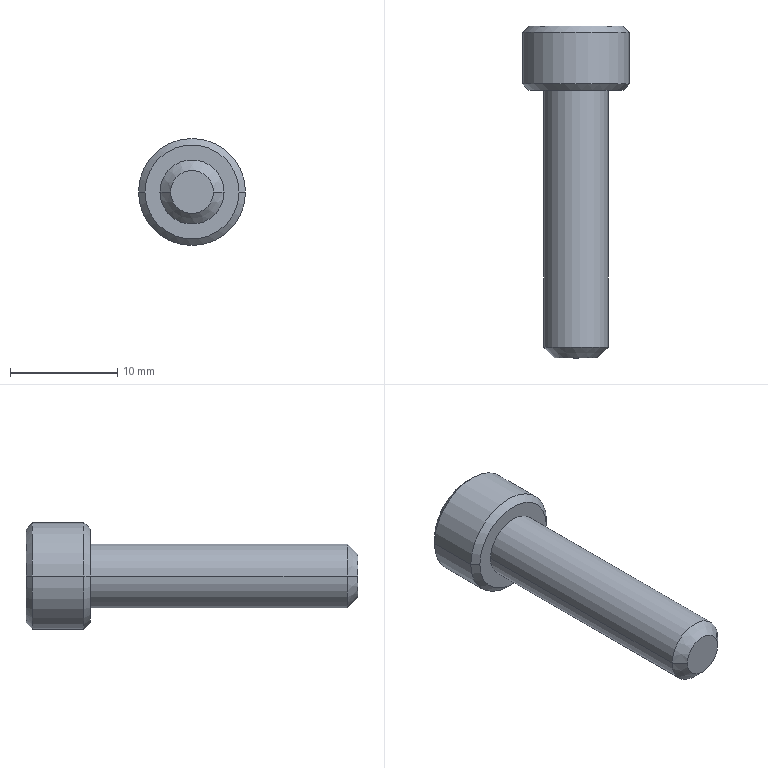Part | STEP file | BB62-M6-25L-1 | 1 solid | 27 faces | box 10 x 31 x 10 mm | volume 1081 mm3 | plane 15 | cone 8 | cylinder 4 | commonest cylinder face diameters 6 x2 10 x2
STEP:
#1=CARTESIAN_POINT('',(0.,1.349,0.));
#2=VERTEX_POINT('',#1);
#3=CARTESIAN_POINT('',(2.86,3.,0.));
#4=VERTEX_POINT('',#3);
#5=CARTESIAN_POINT('',(0.,1.349,0.));
#6=DIRECTION('',(0.866,0.5,0.));
#7=VECTOR('',#6,1000.);
#8=LINE('',#5,#7);
#9=EDGE_CURVE('',#2,#4,#8,.T.);
#10=ORIENTED_EDGE('',*,*,#9,.F.);
#11=CARTESIAN_POINT('',(-2.86,3.,0.));
#12=VERTEX_POINT('',#11);
#13=CARTESIAN_POINT('',(0.,1.349,0.));
#14=DIRECTION('',(-0.866,0.5,0.));
#15=VECTOR('',#14,1000.);
#16=LINE('',#13,#15);
#17=EDGE_CURVE('',#2,#12,#16,.T.);
#18=ORIENTED_EDGE('',*,*,#17,.T.);
#19=CARTESIAN_POINT('',(-2.477,3.,1.43));
#20=VERTEX_POINT('',#19);
#21=CARTESIAN_POINT('',(0.,3.,0.));
#22=DIRECTION('',(0.,-1.,0.));
#23=DIRECTION('',(-1.,0.,0.));
#24=AXIS2_PLACEMENT_3D('',#21,#22,#23);
#25=CIRCLE('',#24,2.86);
#26=EDGE_CURVE('',#20,#12,#25,.T.);
#27=ORIENTED_EDGE('',*,*,#26,.F.);
#28=CARTESIAN_POINT('',(0.,3.,2.86));
#29=VERTEX_POINT('',#28);
#30=CARTESIAN_POINT('',(0.,3.,0.));
#31=DIRECTION('',(0.,-1.,0.));
#32=DIRECTION('',(-1.,0.,0.));
#33=AXIS2_PLACEMENT_3D('',#30,#31,#32);
#34=CIRCLE('',#33,2.86);
#35=EDGE_CURVE('',#29,#20,#34,.T.);
#36=ORIENTED_EDGE('',*,*,#35,.F.);
#37=CARTESIAN_POINT('',(2.477,3.,1.43));
#38=VERTEX_POINT('',#37);
#39=CARTESIAN_POINT('',(0.,3.,0.));
#40=DIRECTION('',(0.,-1.,0.));
#41=DIRECTION('',(-1.,0.,0.));
#42=AXIS2_PLACEMENT_3D('',#39,#40,#41);
#43=CIRCLE('',#42,2.86);
#44=EDGE_CURVE('',#38,#29,#43,.T.);
#45=ORIENTED_EDGE('',*,*,#44,.F.);
#46=CARTESIAN_POINT('',(0.,3.,0.));
#47=DIRECTION('',(0.,-1.,0.));
#48=DIRECTION('',(-1.,0.,0.));
#49=AXIS2_PLACEMENT_3D('',#46,#47,#48);
#50=CIRCLE('',#49,2.86);
#51=EDGE_CURVE('',#4,#38,#50,.T.);
#52=ORIENTED_EDGE('',*,*,#51,.F.);
#53=EDGE_LOOP('',(#10,#18,#27,#36,#45,#52));
#54=FACE_OUTER_BOUND('',#53,.T.);
#55=CARTESIAN_POINT('',(0.,1001.349,0.));
#56=DIRECTION('',(0.,1.,0.));
#57=DIRECTION('',(1.,0.,0.));
#58=AXIS2_PLACEMENT_3D('',#55,#56,#57);
#59=CONICAL_SURFACE('',#58,1732.051,1.047);
#60=ADVANCED_FACE('',(#54),#59,.F.);
#61=CARTESIAN_POINT('',(2.,-25.,0.));
#62=VERTEX_POINT('',#61);
#63=CARTESIAN_POINT('',(-2.,-25.,0.));
#64=VERTEX_POINT('',#63);
#65=CARTESIAN_POINT('',(0.,-25.,0.));
#66=DIRECTION('',(0.,1.,0.));
#67=DIRECTION('',(1.,0.,0.));
#68=AXIS2_PLACEMENT_3D('',#65,#66,#67);
#69=CIRCLE('',#68,2.);
#70=EDGE_CURVE('',#62,#64,#69,.T.);
#71=ORIENTED_EDGE('',*,*,#70,.T.);
#72=CARTESIAN_POINT('',(-3.,-24.,0.));
#73=VERTEX_POINT('',#72);
#74=CARTESIAN_POINT('',(-2.,-25.,0.));
#75=DIRECTION('',(-0.7071,0.7071,0.));
#76=VECTOR('',#75,1000.);
#77=LINE('',#74,#76);
#78=EDGE_CURVE('',#64,#73,#77,.T.);
#79=ORIENTED_EDGE('',*,*,#78,.T.);
#80=CARTESIAN_POINT('',(3.,-24.,0.));
#81=VERTEX_POINT('',#80);
#82=CARTESIAN_POINT('',(0.,-24.,0.));
#83=DIRECTION('',(0.,-1.,0.));
#84=DIRECTION('',(-1.,0.,0.));
#85=AXIS2_PLACEMENT_3D('',#82,#83,#84);
#86=CIRCLE('',#85,3.);
#87=EDGE_CURVE('',#73,#81,#86,.T.);
#88=ORIENTED_EDGE('',*,*,#87,.T.);
#89=CARTESIAN_POINT('',(2.,-25.,0.));
#90=DIRECTION('',(0.7071,0.7071,0.));
#91=VECTOR('',#90,1000.);
#92=LINE('',#89,#91);
#93=EDGE_CURVE('',#62,#81,#92,.T.);
#94=ORIENTED_EDGE('',*,*,#93,.F.);
#95=EDGE_LOOP('',(#71,#79,#88,#94));
#96=FACE_OUTER_BOUND('',#95,.T.);
#97=CARTESIAN_POINT('',(0.,-25.,0.));
#98=DIRECTION('',(0.,1.,0.));
#99=DIRECTION('',(1.,0.,0.));
#100=AXIS2_PLACEMENT_3D('',#97,#98,#99);
#101=CONICAL_SURFACE('',#100,2.,0.7854);
#102=ADVANCED_FACE('',(#96),#101,.T.);
#103=ORIENTED_EDGE('',*,*,#87,.F.);
#104=CARTESIAN_POINT('',(-3.,0.,0.));
#105=VERTEX_POINT('',#104);
#106=CARTESIAN_POINT('',(-3.,-24.,0.));
#107=DIRECTION('',(0.,1.,0.));
#108=VECTOR('',#107,1000.);
#109=LINE('',#106,#108);
#110=EDGE_CURVE('',#73,#105,#109,.T.);
#111=ORIENTED_EDGE('',*,*,#110,.T.);
#112=CARTESIAN_POINT('',(3.,0.,0.));
#113=VERTEX_POINT('',#112);
#114=CARTESIAN_POINT('',(0.,0.,0.));
#115=DIRECTION('',(0.,-1.,0.));
#116=DIRECTION('',(-1.,0.,0.));
#117=AXIS2_PLACEMENT_3D('',#114,#115,#116);
#118=CIRCLE('',#117,3.);
#119=EDGE_CURVE('',#105,#113,#118,.T.);
#120=ORIENTED_EDGE('',*,*,#119,.T.);
#121=CARTESIAN_POINT('',(3.,-24.,0.));
#122=DIRECTION('',(0.,1.,0.));
#123=VECTOR('',#122,1000.);
#124=LINE('',#121,#123);
#125=EDGE_CURVE('',#81,#113,#124,.T.);
#126=ORIENTED_EDGE('',*,*,#125,.F.);
#127=EDGE_LOOP('',(#103,#111,#120,#126));
#128=FACE_OUTER_BOUND('',#127,.T.);
#129=CARTESIAN_POINT('',(0.,-24.,0.));
#130=DIRECTION('',(0.,1.,0.));
#131=DIRECTION('',(1.,0.,0.));
#132=AXIS2_PLACEMENT_3D('',#129,#130,#131);
#133=CYLINDRICAL_SURFACE('',#132,3.);
#134=ADVANCED_FACE('',(#128),#133,.T.);
#135=CARTESIAN_POINT('',(-4.4,6.,0.));
#136=VERTEX_POINT('',#135);
#137=CARTESIAN_POINT('',(4.4,6.,0.));
#138=VERTEX_POINT('',#137);
#139=CARTESIAN_POINT('',(0.,6.,0.));
#140=DIRECTION('',(0.,-1.,0.));
#141=DIRECTION('',(-1.,0.,0.));
#142=AXIS2_PLACEMENT_3D('',#139,#140,#141);
#143=CIRCLE('',#142,4.4);
#144=EDGE_CURVE('',#136,#138,#143,.T.);
#145=ORIENTED_EDGE('',*,*,#144,.T.);
#146=CARTESIAN_POINT('',(5.,5.4,0.));
#147=VERTEX_POINT('',#146);
#148=CARTESIAN_POINT('',(5.,5.4,0.));
#149=DIRECTION('',(0.7071,-0.7071,0.));
#150=VECTOR('',#149,1000.);
#151=LINE('',#148,#150);
#152=EDGE_CURVE('',#138,#147,#151,.T.);
#153=ORIENTED_EDGE('',*,*,#152,.T.);
#154=CARTESIAN_POINT('',(-5.,5.4,0.));
#155=VERTEX_POINT('',#154);
#156=CARTESIAN_POINT('',(0.,5.4,0.));
#157=DIRECTION('',(0.,-1.,0.));
#158=DIRECTION('',(-1.,0.,0.));
#159=AXIS2_PLACEMENT_3D('',#156,#157,#158);
#160=CIRCLE('',#159,5.);
#161=EDGE_CURVE('',#155,#147,#160,.T.);
#162=ORIENTED_EDGE('',*,*,#161,.F.);
#163=CARTESIAN_POINT('',(-5.,5.4,0.));
#164=DIRECTION('',(-0.7071,-0.7071,0.));
#165=VECTOR('',#164,1000.);
#166=LINE('',#163,#165);
#167=EDGE_CURVE('',#136,#155,#166,.T.);
#168=ORIENTED_EDGE('',*,*,#167,.F.);
#169=EDGE_LOOP('',(#145,#153,#162,#168));
#170=FACE_OUTER_BOUND('',#169,.T.);
#171=CARTESIAN_POINT('',(0.,5.4,0.));
#172=DIRECTION('',(0.,-1.,0.));
#173=DIRECTION('',(-1.,0.,0.));
#174=AXIS2_PLACEMENT_3D('',#171,#172,#173);
#175=CONICAL_SURFACE('',#174,5.,0.7854);
#176=ADVANCED_FACE('',(#170),#175,.T.);
#177=ORIENTED_EDGE('',*,*,#161,.T.);
#178=CARTESIAN_POINT('',(5.,0.6,0.));
#179=VERTEX_POINT('',#178);
#180=CARTESIAN_POINT('',(5.,1.62,0.));
#181=DIRECTION('',(0.,-1.,0.));
#182=VECTOR('',#181,1000.);
#183=LINE('',#180,#182);
#184=EDGE_CURVE('',#147,#179,#183,.T.);
#185=ORIENTED_EDGE('',*,*,#184,.T.);
#186=CARTESIAN_POINT('',(-5.,0.6,0.));
#187=VERTEX_POINT('',#186);
#188=CARTESIAN_POINT('',(0.,0.6,0.));
#189=DIRECTION('',(0.,-1.,0.));
#190=DIRECTION('',(-1.,0.,0.));
#191=AXIS2_PLACEMENT_3D('',#188,#189,#190);
#192=CIRCLE('',#191,5.);
#193=EDGE_CURVE('',#187,#179,#192,.T.);
#194=ORIENTED_EDGE('',*,*,#193,.F.);
#195=CARTESIAN_POINT('',(-5.,1.62,0.));
#196=DIRECTION('',(0.,-1.,0.));
#197=VECTOR('',#196,1000.);
#198=LINE('',#195,#197);
#199=EDGE_CURVE('',#155,#187,#198,.T.);
#200=ORIENTED_EDGE('',*,*,#199,.F.);
#201=EDGE_LOOP('',(#177,#185,#194,#200));
#202=FACE_OUTER_BOUND('',#201,.T.);
#203=CARTESIAN_POINT('',(0.,1.62,0.));
#204=DIRECTION('',(0.,-1.,0.));
#205=DIRECTION('',(-1.,0.,0.));
#206=AXIS2_PLACEMENT_3D('',#203,#204,#205);
#207=CYLINDRICAL_SURFACE('',#206,5.);
#208=ADVANCED_FACE('',(#202),#207,.T.);
#209=CARTESIAN_POINT('',(-4.4,0.,0.));
#210=VERTEX_POINT('',#209);
#211=CARTESIAN_POINT('',(4.4,0.,0.));
#212=VERTEX_POINT('',#211);
#213=CARTESIAN_POINT('',(0.,0.,0.));
#214=DIRECTION('',(0.,-1.,0.));
#215=DIRECTION('',(-1.,0.,0.));
#216=AXIS2_PLACEMENT_3D('',#213,#214,#215);
#217=CIRCLE('',#216,4.4);
#218=EDGE_CURVE('',#210,#212,#217,.T.);
#219=ORIENTED_EDGE('',*,*,#218,.F.);
#220=CARTESIAN_POINT('',(-4.4,0.,0.));
#221=DIRECTION('',(-0.7071,0.7071,0.));
#222=VECTOR('',#221,1000.);
#223=LINE('',#220,#222);
#224=EDGE_CURVE('',#210,#187,#223,.T.);
#225=ORIENTED_EDGE('',*,*,#224,.T.);
#226=ORIENTED_EDGE('',*,*,#193,.T.);
#227=CARTESIAN_POINT('',(4.4,0.,0.));
#228=DIRECTION('',(0.7071,0.7071,0.));
#229=VECTOR('',#228,1000.);
#230=LINE('',#227,#229);
#231=EDGE_CURVE('',#212,#179,#230,.T.);
#232=ORIENTED_EDGE('',*,*,#231,.F.);
#233=EDGE_LOOP('',(#219,#225,#226,#232));
#234=FACE_OUTER_BOUND('',#233,.T.);
#235=CARTESIAN_POINT('',(0.,0.,0.));
#236=DIRECTION('',(0.,1.,0.));
#237=DIRECTION('',(1.,0.,0.));
#238=AXIS2_PLACEMENT_3D('',#235,#236,#237);
#239=CONICAL_SURFACE('',#238,4.4,0.7854);
#240=ADVANCED_FACE('',(#234),#239,.T.);
#241=ORIENTED_EDGE('',*,*,#144,.F.);
#242=CARTESIAN_POINT('',(0.,6.,0.));
#243=DIRECTION('',(0.,-1.,0.));
#244=DIRECTION('',(-1.,0.,0.));
#245=AXIS2_PLACEMENT_3D('',#242,#243,#244);
#246=CIRCLE('',#245,4.4);
#247=EDGE_CURVE('',#138,#136,#246,.T.);
#248=ORIENTED_EDGE('',*,*,#247,.F.);
#249=EDGE_LOOP('',(#241,#248));
#250=FACE_OUTER_BOUND('',#249,.T.);
#251=CARTESIAN_POINT('',(0.,6.,-2.86));
#252=VERTEX_POINT('',#251);
#253=CARTESIAN_POINT('',(-2.477,6.,-1.43));
#254=VERTEX_POINT('',#253);
#255=CARTESIAN_POINT('',(0.,6.,-2.86));
#256=DIRECTION('',(-0.866,0.,0.5));
#257=VECTOR('',#256,1000.);
#258=LINE('',#255,#257);
#259=EDGE_CURVE('',#252,#254,#258,.T.);
#260=ORIENTED_EDGE('',*,*,#259,.F.);
#261=CARTESIAN_POINT('',(2.477,6.,-1.43));
#262=VERTEX_POINT('',#261);
#263=CARTESIAN_POINT('',(2.477,6.,-1.43));
#264=DIRECTION('',(-0.866,0.,-0.5));
#265=VECTOR('',#264,1000.);
#266=LINE('',#263,#265);
#267=EDGE_CURVE('',#262,#252,#266,.T.);
#268=ORIENTED_EDGE('',*,*,#267,.F.);
#269=CARTESIAN_POINT('',(2.477,6.,1.43));
#270=VERTEX_POINT('',#269);
#271=CARTESIAN_POINT('',(2.477,6.,1.43));
#272=DIRECTION('',(0.,0.,-1.));
#273=VECTOR('',#272,1000.);
#274=LINE('',#271,#273);
#275=EDGE_CURVE('',#270,#262,#274,.T.);
#276=ORIENTED_EDGE('',*,*,#275,.F.);
#277=CARTESIAN_POINT('',(0.,6.,2.86));
#278=VERTEX_POINT('',#277);
#279=CARTESIAN_POINT('',(0.,6.,2.86));
#280=DIRECTION('',(0.866,0.,-0.5));
#281=VECTOR('',#280,1000.);
#282=LINE('',#279,#281);
#283=EDGE_CURVE('',#278,#270,#282,.T.);
#284=ORIENTED_EDGE('',*,*,#283,.F.);
#285=CARTESIAN_POINT('',(-2.477,6.,1.43));
#286=VERTEX_POINT('',#285);
#287=CARTESIAN_POINT('',(-2.477,6.,1.43));
#288=DIRECTION('',(0.866,0.,0.5));
#289=VECTOR('',#288,1000.);
#290=LINE('',#287,#289);
#291=EDGE_CURVE('',#286,#278,#290,.T.);
#292=ORIENTED_EDGE('',*,*,#291,.F.);
#293=CARTESIAN_POINT('',(-2.477,6.,-1.43));
#294=DIRECTION('',(0.,0.,1.));
#295=VECTOR('',#294,1000.);
#296=LINE('',#293,#295);
#297=EDGE_CURVE('',#254,#286,#296,.T.);
#298=ORIENTED_EDGE('',*,*,#297,.F.);
#299=EDGE_LOOP('',(#260,#268,#276,#284,#292,#298));
#300=FACE_BOUND('',#299,.T.);
#301=CARTESIAN_POINT('',(4.4,6.,0.));
#302=DIRECTION('',(0.,1.,0.));
#303=DIRECTION('',(1.,0.,0.));
#304=AXIS2_PLACEMENT_3D('',#301,#302,#303);
#305=PLANE('',#304);
#306=ADVANCED_FACE('',(#250,#300),#305,.T.);
#307=CARTESIAN_POINT('',(0.,0.,0.));
#308=DIRECTION('',(0.,-1.,0.));
#309=DIRECTION('',(-1.,0.,0.));
#310=AXIS2_PLACEMENT_3D('',#307,#308,#309);
#311=CIRCLE('',#310,3.);
#312=EDGE_CURVE('',#113,#105,#311,.T.);
#313=ORIENTED_EDGE('',*,*,#312,.F.);
#314=ORIENTED_EDGE('',*,*,#119,.F.);
#315=EDGE_LOOP('',(#313,#314));
#316=FACE_BOUND('',#315,.T.);
#317=CARTESIAN_POINT('',(0.,0.,0.));
#318=DIRECTION('',(0.,-1.,0.));
#319=DIRECTION('',(-1.,0.,0.));
#320=AXIS2_PLACEMENT_3D('',#317,#318,#319);
#321=CIRCLE('',#320,4.4);
#322=EDGE_CURVE('',#212,#210,#321,.T.);
#323=ORIENTED_EDGE('',*,*,#322,.T.);
#324=ORIENTED_EDGE('',*,*,#218,.T.);
#325=EDGE_LOOP('',(#323,#324));
#326=FACE_OUTER_BOUND('',#325,.T.);
#327=CARTESIAN_POINT('',(0.,0.,0.));
#328=DIRECTION('',(0.,-1.,0.));
#329=DIRECTION('',(-1.,0.,0.));
#330=AXIS2_PLACEMENT_3D('',#327,#328,#329);
#331=PLANE('',#330);
#332=ADVANCED_FACE('',(#316,#326),#331,.T.);
#333=ORIENTED_EDGE('',*,*,#224,.F.);
#334=ORIENTED_EDGE('',*,*,#322,.F.);
#335=ORIENTED_EDGE('',*,*,#231,.T.);
#336=CARTESIAN_POINT('',(0.,0.6,0.));
#337=DIRECTION('',(0.,-1.,0.));
#338=DIRECTION('',(-1.,0.,0.));
#339=AXIS2_PLACEMENT_3D('',#336,#337,#338);
#340=CIRCLE('',#339,5.);
#341=EDGE_CURVE('',#179,#187,#340,.T.);
#342=ORIENTED_EDGE('',*,*,#341,.T.);
#343=EDGE_LOOP('',(#333,#334,#335,#342));
#344=FACE_OUTER_BOUND('',#343,.T.);
#345=CARTESIAN_POINT('',(0.,0.,0.));
#346=DIRECTION('',(0.,1.,0.));
#347=DIRECTION('',(1.,0.,0.));
#348=AXIS2_PLACEMENT_3D('',#345,#346,#347);
#349=CONICAL_SURFACE('',#348,4.4,0.7854);
#350=ADVANCED_FACE('',(#344),#349,.T.);
#351=ORIENTED_EDGE('',*,*,#184,.F.);
#352=CARTESIAN_POINT('',(0.,5.4,0.));
#353=DIRECTION('',(0.,-1.,0.));
#354=DIRECTION('',(-1.,0.,0.));
#355=AXIS2_PLACEMENT_3D('',#352,#353,#354);
#356=CIRCLE('',#355,5.);
#357=EDGE_CURVE('',#147,#155,#356,.T.);
#358=ORIENTED_EDGE('',*,*,#357,.T.);
#359=ORIENTED_EDGE('',*,*,#199,.T.);
#360=ORIENTED_EDGE('',*,*,#341,.F.);
#361=EDGE_LOOP('',(#351,#358,#359,#360));
#362=FACE_OUTER_BOUND('',#361,.T.);
#363=CARTESIAN_POINT('',(0.,1.62,0.));
#364=DIRECTION('',(0.,-1.,0.));
#365=DIRECTION('',(-1.,0.,0.));
#366=AXIS2_PLACEMENT_3D('',#363,#364,#365);
#367=CYLINDRICAL_SURFACE('',#366,5.);
#368=ADVANCED_FACE('',(#362),#367,.T.);
#369=ORIENTED_EDGE('',*,*,#152,.F.);
#370=ORIENTED_EDGE('',*,*,#247,.T.);
#371=ORIENTED_EDGE('',*,*,#167,.T.);
#372=ORIENTED_EDGE('',*,*,#357,.F.);
#373=EDGE_LOOP('',(#369,#370,#371,#372));
#374=FACE_OUTER_BOUND('',#373,.T.);
#375=CARTESIAN_POINT('',(0.,5.4,0.));
#376=DIRECTION('',(0.,-1.,0.));
#377=DIRECTION('',(-1.,0.,0.));
#378=AXIS2_PLACEMENT_3D('',#375,#376,#377);
#379=CONICAL_SURFACE('',#378,5.,0.7854);
#380=ADVANCED_FACE('',(#374),#379,.T.);
#381=ORIENTED_EDGE('',*,*,#110,.F.);
#382=CARTESIAN_POINT('',(0.,-24.,0.));
#383=DIRECTION('',(0.,-1.,0.));
#384=DIRECTION('',(-1.,0.,0.));
#385=AXIS2_PLACEMENT_3D('',#382,#383,#384);
#386=CIRCLE('',#385,3.);
#387=EDGE_CURVE('',#81,#73,#386,.T.);
#388=ORIENTED_EDGE('',*,*,#387,.F.);
#389=ORIENTED_EDGE('',*,*,#125,.T.);
#390=ORIENTED_EDGE('',*,*,#312,.T.);
#391=EDGE_LOOP('',(#381,#388,#389,#390));
#392=FACE_OUTER_BOUND('',#391,.T.);
#393=CARTESIAN_POINT('',(0.,-24.,0.));
#394=DIRECTION('',(0.,1.,0.));
#395=DIRECTION('',(1.,0.,0.));
#396=AXIS2_PLACEMENT_3D('',#393,#394,#395);
#397=CYLINDRICAL_SURFACE('',#396,3.);
#398=ADVANCED_FACE('',(#392),#397,.T.);
#399=ORIENTED_EDGE('',*,*,#70,.F.);
#400=CARTESIAN_POINT('',(0.,-25.,0.));
#401=DIRECTION('',(0.,1.,0.));
#402=DIRECTION('',(1.,0.,0.));
#403=AXIS2_PLACEMENT_3D('',#400,#401,#402);
#404=CIRCLE('',#403,2.);
#405=EDGE_CURVE('',#64,#62,#404,.T.);
#406=ORIENTED_EDGE('',*,*,#405,.F.);
#407=EDGE_LOOP('',(#399,#406));
#408=FACE_OUTER_BOUND('',#407,.T.);
#409=CARTESIAN_POINT('',(0.,-25.,0.));
#410=DIRECTION('',(0.,-1.,0.));
#411=DIRECTION('',(-1.,0.,0.));
#412=AXIS2_PLACEMENT_3D('',#409,#410,#411);
#413=PLANE('',#412);
#414=ADVANCED_FACE('',(#408),#413,.T.);
#415=ORIENTED_EDGE('',*,*,#78,.F.);
#416=ORIENTED_EDGE('',*,*,#405,.T.);
#417=ORIENTED_EDGE('',*,*,#93,.T.);
#418=ORIENTED_EDGE('',*,*,#387,.T.);
#419=EDGE_LOOP('',(#415,#416,#417,#418));
#420=FACE_OUTER_BOUND('',#419,.T.);
#421=CARTESIAN_POINT('',(0.,-25.,0.));
#422=DIRECTION('',(0.,1.,0.));
#423=DIRECTION('',(1.,0.,0.));
#424=AXIS2_PLACEMENT_3D('',#421,#422,#423);
#425=CONICAL_SURFACE('',#424,2.,0.7854);
#426=ADVANCED_FACE('',(#420),#425,.T.);
#427=CARTESIAN_POINT('',(2.477,3.,-1.43));
#428=VERTEX_POINT('',#427);
#429=CARTESIAN_POINT('',(0.,3.,-2.86));
#430=VERTEX_POINT('',#429);
#431=CARTESIAN_POINT('',(2.477,3.,-1.43));
#432=DIRECTION('',(-0.866,0.,-0.5));
#433=VECTOR('',#432,1000.);
#434=LINE('',#431,#433);
#435=EDGE_CURVE('',#428,#430,#434,.T.);
#436=ORIENTED_EDGE('',*,*,#435,.F.);
#437=CARTESIAN_POINT('',(2.477,6.,-1.43));
#438=DIRECTION('',(0.,-1.,0.));
#439=VECTOR('',#438,1000.);
#440=LINE('',#437,#439);
#441=EDGE_CURVE('',#262,#428,#440,.T.);
#442=ORIENTED_EDGE('',*,*,#441,.F.);
#443=ORIENTED_EDGE('',*,*,#267,.T.);
#444=CARTESIAN_POINT('',(0.,6.,-2.86));
#445=DIRECTION('',(0.,-1.,0.));
#446=VECTOR('',#445,1000.);
#447=LINE('',#444,#446);
#448=EDGE_CURVE('',#252,#430,#447,.T.);
#449=ORIENTED_EDGE('',*,*,#448,.T.);
#450=EDGE_LOOP('',(#436,#442,#443,#449));
#451=FACE_OUTER_BOUND('',#450,.T.);
#452=CARTESIAN_POINT('',(2.477,6.,-1.43));
#453=DIRECTION('',(-0.5,0.,0.866));
#454=DIRECTION('',(0.866,0.,0.5));
#455=AXIS2_PLACEMENT_3D('',#452,#453,#454);
#456=PLANE('',#455);
#457=ADVANCED_FACE('',(#451),#456,.T.);
#458=CARTESIAN_POINT('',(-2.477,3.,-1.43));
#459=VERTEX_POINT('',#458);
#460=CARTESIAN_POINT('',(0.,3.,-2.86));
#461=DIRECTION('',(-0.866,0.,0.5));
#462=VECTOR('',#461,1000.);
#463=LINE('',#460,#462);
#464=EDGE_CURVE('',#430,#459,#463,.T.);
#465=ORIENTED_EDGE('',*,*,#464,.F.);
#466=ORIENTED_EDGE('',*,*,#448,.F.);
#467=ORIENTED_EDGE('',*,*,#259,.T.);
#468=CARTESIAN_POINT('',(-2.477,6.,-1.43));
#469=DIRECTION('',(0.,-1.,0.));
#470=VECTOR('',#469,1000.);
#471=LINE('',#468,#470);
#472=EDGE_CURVE('',#254,#459,#471,.T.);
#473=ORIENTED_EDGE('',*,*,#472,.T.);
#474=EDGE_LOOP('',(#465,#466,#467,#473));
#475=FACE_OUTER_BOUND('',#474,.T.);
#476=CARTESIAN_POINT('',(0.,6.,-2.86));
#477=DIRECTION('',(0.5,0.,0.866));
#478=DIRECTION('',(0.866,0.,-0.5));
#479=AXIS2_PLACEMENT_3D('',#476,#477,#478);
#480=PLANE('',#479);
#481=ADVANCED_FACE('',(#475),#480,.T.);
#482=CARTESIAN_POINT('',(-2.477,3.,-1.43));
#483=DIRECTION('',(0.,0.,1.));
#484=VECTOR('',#483,1000.);
#485=LINE('',#482,#484);
#486=EDGE_CURVE('',#459,#20,#485,.T.);
#487=ORIENTED_EDGE('',*,*,#486,.F.);
#488=ORIENTED_EDGE('',*,*,#472,.F.);
#489=ORIENTED_EDGE('',*,*,#297,.T.);
#490=CARTESIAN_POINT('',(-2.477,6.,1.43));
#491=DIRECTION('',(0.,-1.,0.));
#492=VECTOR('',#491,1000.);
#493=LINE('',#490,#492);
#494=EDGE_CURVE('',#286,#20,#493,.T.);
#495=ORIENTED_EDGE('',*,*,#494,.T.);
#496=EDGE_LOOP('',(#487,#488,#489,#495));
#497=FACE_OUTER_BOUND('',#496,.T.);
#498=CARTESIAN_POINT('',(-2.477,6.,-1.43));
#499=DIRECTION('',(1.,0.,0.));
#500=DIRECTION('',(0.,0.,-1.));
#501=AXIS2_PLACEMENT_3D('',#498,#499,#500);
#502=PLANE('',#501);
#503=ADVANCED_FACE('',(#497),#502,.T.);
#504=CARTESIAN_POINT('',(-2.477,3.,1.43));
#505=DIRECTION('',(0.866,0.,0.5));
#506=VECTOR('',#505,1000.);
#507=LINE('',#504,#506);
#508=EDGE_CURVE('',#20,#29,#507,.T.);
#509=ORIENTED_EDGE('',*,*,#508,.F.);
#510=ORIENTED_EDGE('',*,*,#494,.F.);
#511=ORIENTED_EDGE('',*,*,#291,.T.);
#512=CARTESIAN_POINT('',(0.,6.,2.86));
#513=DIRECTION('',(0.,-1.,0.));
#514=VECTOR('',#513,1000.);
#515=LINE('',#512,#514);
#516=EDGE_CURVE('',#278,#29,#515,.T.);
#517=ORIENTED_EDGE('',*,*,#516,.T.);
#518=EDGE_LOOP('',(#509,#510,#511,#517));
#519=FACE_OUTER_BOUND('',#518,.T.);
#520=CARTESIAN_POINT('',(-2.477,6.,1.43));
#521=DIRECTION('',(0.5,0.,-0.866));
#522=DIRECTION('',(-0.866,0.,-0.5));
#523=AXIS2_PLACEMENT_3D('',#520,#521,#522);
#524=PLANE('',#523);
#525=ADVANCED_FACE('',(#519),#524,.T.);
#526=CARTESIAN_POINT('',(0.,3.,2.86));
#527=DIRECTION('',(0.866,0.,-0.5));
#528=VECTOR('',#527,1000.);
#529=LINE('',#526,#528);
#530=EDGE_CURVE('',#29,#38,#529,.T.);
#531=ORIENTED_EDGE('',*,*,#530,.F.);
#532=ORIENTED_EDGE('',*,*,#516,.F.);
#533=ORIENTED_EDGE('',*,*,#283,.T.);
#534=CARTESIAN_POINT('',(2.477,6.,1.43));
#535=DIRECTION('',(0.,-1.,0.));
#536=VECTOR('',#535,1000.);
#537=LINE('',#534,#536);
#538=EDGE_CURVE('',#270,#38,#537,.T.);
#539=ORIENTED_EDGE('',*,*,#538,.T.);
#540=EDGE_LOOP('',(#531,#532,#533,#539));
#541=FACE_OUTER_BOUND('',#540,.T.);
#542=CARTESIAN_POINT('',(0.,6.,2.86));
#543=DIRECTION('',(-0.5,0.,-0.866));
#544=DIRECTION('',(-0.866,0.,0.5));
#545=AXIS2_PLACEMENT_3D('',#542,#543,#544);
#546=PLANE('',#545);
#547=ADVANCED_FACE('',(#541),#546,.T.);
#548=CARTESIAN_POINT('',(2.477,3.,1.43));
#549=DIRECTION('',(0.,0.,-1.));
#550=VECTOR('',#549,1000.);
#551=LINE('',#548,#550);
#552=EDGE_CURVE('',#38,#428,#551,.T.);
#553=ORIENTED_EDGE('',*,*,#552,.F.);
#554=ORIENTED_EDGE('',*,*,#538,.F.);
#555=ORIENTED_EDGE('',*,*,#275,.T.);
#556=ORIENTED_EDGE('',*,*,#441,.T.);
#557=EDGE_LOOP('',(#553,#554,#555,#556));
#558=FACE_OUTER_BOUND('',#557,.T.);
#559=CARTESIAN_POINT('',(2.477,6.,1.43));
#560=DIRECTION('',(-1.,0.,0.));
#561=DIRECTION('',(0.,0.,1.));
#562=AXIS2_PLACEMENT_3D('',#559,#560,#561);
#563=PLANE('',#562);
#564=ADVANCED_FACE('',(#558),#563,.T.);
#565=ORIENTED_EDGE('',*,*,#435,.T.);
#566=CARTESIAN_POINT('',(0.,3.,0.));
#567=DIRECTION('',(0.,-1.,0.));
#568=DIRECTION('',(-1.,0.,0.));
#569=AXIS2_PLACEMENT_3D('',#566,#567,#568);
#570=CIRCLE('',#569,2.86);
#571=EDGE_CURVE('',#430,#428,#570,.T.);
#572=ORIENTED_EDGE('',*,*,#571,.T.);
#573=EDGE_LOOP('',(#565,#572));
#574=FACE_OUTER_BOUND('',#573,.T.);
#575=CARTESIAN_POINT('',(0.,3.,0.));
#576=DIRECTION('',(0.,1.,0.));
#577=DIRECTION('',(1.,0.,0.));
#578=AXIS2_PLACEMENT_3D('',#575,#576,#577);
#579=PLANE('',#578);
#580=ADVANCED_FACE('',(#574),#579,.F.);
#581=ORIENTED_EDGE('',*,*,#552,.T.);
#582=CARTESIAN_POINT('',(0.,3.,0.));
#583=DIRECTION('',(0.,-1.,0.));
#584=DIRECTION('',(-1.,0.,0.));
#585=AXIS2_PLACEMENT_3D('',#582,#583,#584);
#586=CIRCLE('',#585,2.86);
#587=EDGE_CURVE('',#428,#4,#586,.T.);
#588=ORIENTED_EDGE('',*,*,#587,.T.);
#589=ORIENTED_EDGE('',*,*,#51,.T.);
#590=EDGE_LOOP('',(#581,#588,#589));
#591=FACE_OUTER_BOUND('',#590,.T.);
#592=CARTESIAN_POINT('',(0.,3.,0.));
#593=DIRECTION('',(0.,1.,0.));
#594=DIRECTION('',(1.,0.,0.));
#595=AXIS2_PLACEMENT_3D('',#592,#593,#594);
#596=PLANE('',#595);
#597=ADVANCED_FACE('',(#591),#596,.F.);
#598=ORIENTED_EDGE('',*,*,#530,.T.);
#599=ORIENTED_EDGE('',*,*,#44,.T.);
#600=EDGE_LOOP('',(#598,#599));
#601=FACE_OUTER_BOUND('',#600,.T.);
#602=CARTESIAN_POINT('',(0.,3.,0.));
#603=DIRECTION('',(0.,1.,0.));
#604=DIRECTION('',(1.,0.,0.));
#605=AXIS2_PLACEMENT_3D('',#602,#603,#604);
#606=PLANE('',#605);
#607=ADVANCED_FACE('',(#601),#606,.F.);
#608=ORIENTED_EDGE('',*,*,#508,.T.);
#609=ORIENTED_EDGE('',*,*,#35,.T.);
#610=EDGE_LOOP('',(#608,#609));
#611=FACE_OUTER_BOUND('',#610,.T.);
#612=CARTESIAN_POINT('',(0.,3.,0.));
#613=DIRECTION('',(0.,1.,0.));
#614=DIRECTION('',(1.,0.,0.));
#615=AXIS2_PLACEMENT_3D('',#612,#613,#614);
#616=PLANE('',#615);
#617=ADVANCED_FACE('',(#611),#616,.F.);
#618=ORIENTED_EDGE('',*,*,#486,.T.);
#619=ORIENTED_EDGE('',*,*,#26,.T.);
#620=CARTESIAN_POINT('',(0.,3.,0.));
#621=DIRECTION('',(0.,-1.,0.));
#622=DIRECTION('',(-1.,0.,0.));
#623=AXIS2_PLACEMENT_3D('',#620,#621,#622);
#624=CIRCLE('',#623,2.86);
#625=EDGE_CURVE('',#12,#459,#624,.T.);
#626=ORIENTED_EDGE('',*,*,#625,.T.);
#627=EDGE_LOOP('',(#618,#619,#626));
#628=FACE_OUTER_BOUND('',#627,.T.);
#629=CARTESIAN_POINT('',(0.,3.,0.));
#630=DIRECTION('',(0.,1.,0.));
#631=DIRECTION('',(1.,0.,0.));
#632=AXIS2_PLACEMENT_3D('',#629,#630,#631);
#633=PLANE('',#632);
#634=ADVANCED_FACE('',(#628),#633,.F.);
#635=ORIENTED_EDGE('',*,*,#464,.T.);
#636=CARTESIAN_POINT('',(0.,3.,0.));
#637=DIRECTION('',(0.,-1.,0.));
#638=DIRECTION('',(-1.,0.,0.));
#639=AXIS2_PLACEMENT_3D('',#636,#637,#638);
#640=CIRCLE('',#639,2.86);
#641=EDGE_CURVE('',#459,#430,#640,.T.);
#642=ORIENTED_EDGE('',*,*,#641,.T.);
#643=EDGE_LOOP('',(#635,#642));
#644=FACE_OUTER_BOUND('',#643,.T.);
#645=CARTESIAN_POINT('',(0.,3.,0.));
#646=DIRECTION('',(0.,1.,0.));
#647=DIRECTION('',(1.,0.,0.));
#648=AXIS2_PLACEMENT_3D('',#645,#646,#647);
#649=PLANE('',#648);
#650=ADVANCED_FACE('',(#644),#649,.F.);
#651=ORIENTED_EDGE('',*,*,#17,.F.);
#652=ORIENTED_EDGE('',*,*,#9,.T.);
#653=ORIENTED_EDGE('',*,*,#587,.F.);
#654=ORIENTED_EDGE('',*,*,#571,.F.);
#655=ORIENTED_EDGE('',*,*,#641,.F.);
#656=ORIENTED_EDGE('',*,*,#625,.F.);
#657=EDGE_LOOP('',(#651,#652,#653,#654,#655,#656));
#658=FACE_OUTER_BOUND('',#657,.T.);
#659=CARTESIAN_POINT('',(0.,1001.349,0.));
#660=DIRECTION('',(0.,1.,0.));
#661=DIRECTION('',(1.,0.,0.));
#662=AXIS2_PLACEMENT_3D('',#659,#660,#661);
#663=CONICAL_SURFACE('',#662,1732.051,1.047);
#664=ADVANCED_FACE('',(#658),#663,.F.);
#665=CLOSED_SHELL('',(#60,#102,#134,#176,#208,#240,#306,#332,#350,#368,#380,#398,#414,#426,#457,#481,#503,#525,#547,#564,#580,#597,#607,#617,#634,#650,#664));
#666=MANIFOLD_SOLID_BREP('',#665);
#667=CARTESIAN_POINT('',(0.,0.,0.));
#668=DIRECTION('',(0.,0.,1.));
#669=DIRECTION('',(1.,0.,0.));
#670=AXIS2_PLACEMENT_3D('',#667,#668,#669);
#671=(LENGTH_UNIT()NAMED_UNIT(*)SI_UNIT(.MILLI.,.METRE.));
#672=UNCERTAINTY_MEASURE_WITH_UNIT(LENGTH_MEASURE(0.00001),#671,'','');
#673=(NAMED_UNIT(*)PLANE_ANGLE_UNIT()SI_UNIT($,.RADIAN.));
#674=(NAMED_UNIT(*)SI_UNIT($,.STERADIAN.)SOLID_ANGLE_UNIT());
#675=(GEOMETRIC_REPRESENTATION_CONTEXT(3)GLOBAL_UNCERTAINTY_ASSIGNED_CONTEXT((#672))GLOBAL_UNIT_ASSIGNED_CONTEXT((#671,#673,#674))REPRESENTATION_CONTEXT('',''));
#676=ADVANCED_BREP_SHAPE_REPRESENTATION('',(#666,#670),#675);